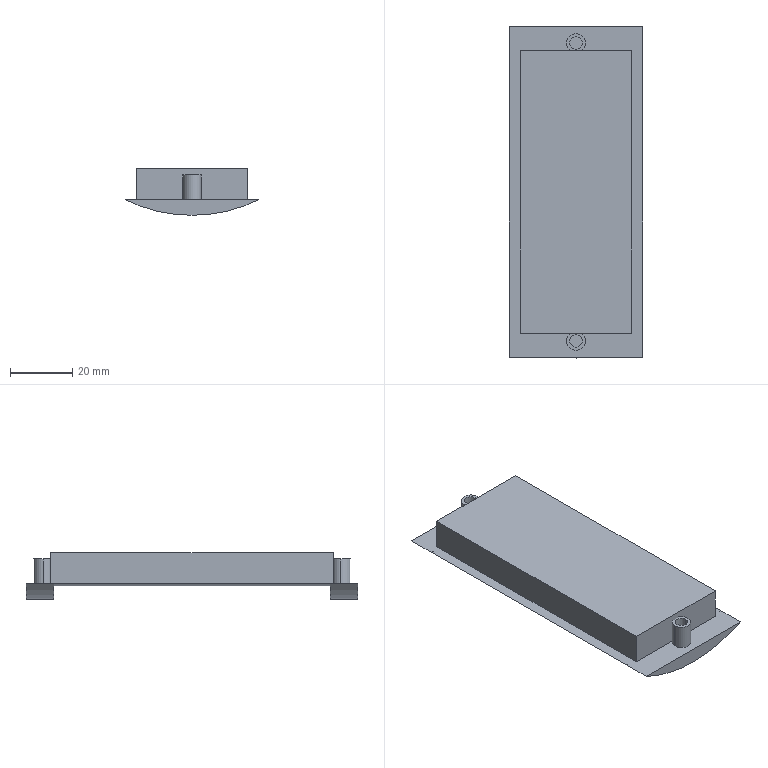Part | STEP file | GY-AA29-AL06-96 nylon handle | 3 solids | 36 faces | box 43 x 107 x 15 mm | volume 16385 mm3 | cylinder 19 | plane 17 | commonest cylinder face diameters 4 x4 6 x4 97.45 x4 10 x3 19.866 x2 56.416 x2